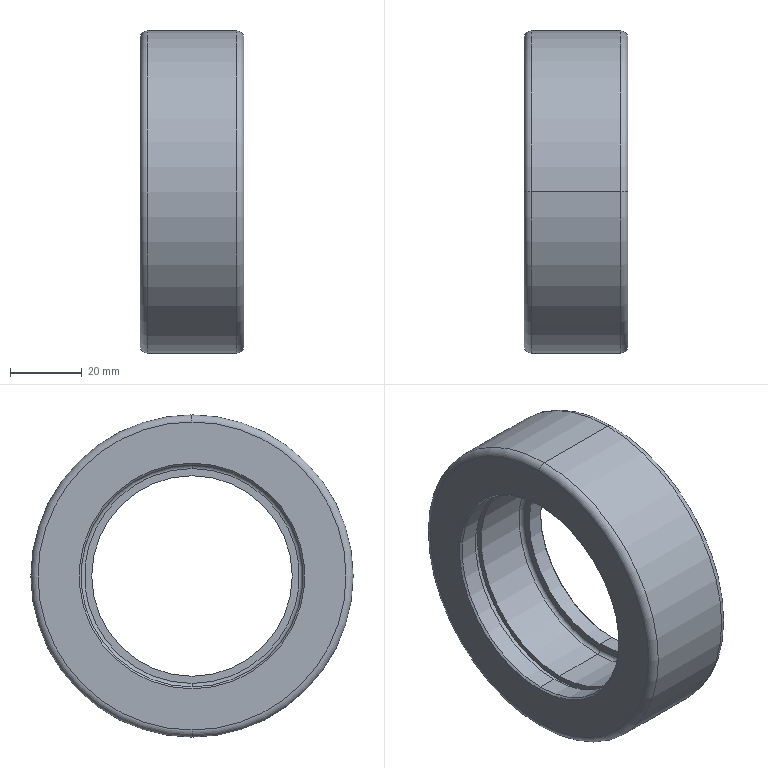Part | STEP file | PN_0001-01-11 Guide wheel B | 1 solid | 25 faces | box 29 x 90 x 90 mm | volume 98573 mm3 | cylinder 10 | torus 6 | plane 5 | cone 4 | commonest cylinder face diameters 62 x4 56 x2 65 x2 90 x2
STEP:
#1=CARTESIAN_POINT('',(0.5,0.,-31.));
#2=VERTEX_POINT('',#1);
#3=CARTESIAN_POINT('',(0.5,0.,31.));
#4=VERTEX_POINT('',#3);
#5=CARTESIAN_POINT('',(0.5,0.,0.));
#6=DIRECTION('',(-1.,0.,0.));
#7=DIRECTION('',(0.,0.,-1.));
#8=AXIS2_PLACEMENT_3D('',#5,#6,#7);
#9=CIRCLE('',#8,31.);
#10=EDGE_CURVE('',#2,#4,#9,.T.);
#11=ORIENTED_EDGE('',*,*,#10,.F.);
#12=CARTESIAN_POINT('',(0.,0.,-31.5));
#13=VERTEX_POINT('',#12);
#14=CARTESIAN_POINT('',(0.5,0.,-31.));
#15=DIRECTION('',(-0.7071,0.,-0.7071));
#16=VECTOR('',#15,1000.);
#17=LINE('',#14,#16);
#18=EDGE_CURVE('',#2,#13,#17,.T.);
#19=ORIENTED_EDGE('',*,*,#18,.T.);
#20=CARTESIAN_POINT('',(0.,0.,31.5));
#21=VERTEX_POINT('',#20);
#22=CARTESIAN_POINT('',(0.,0.,0.));
#23=DIRECTION('',(1.,0.,0.));
#24=DIRECTION('',(0.,0.,-1.));
#25=AXIS2_PLACEMENT_3D('',#22,#23,#24);
#26=CIRCLE('',#25,31.5);
#27=EDGE_CURVE('',#21,#13,#26,.T.);
#28=ORIENTED_EDGE('',*,*,#27,.F.);
#29=CARTESIAN_POINT('',(0.5,0.,31.));
#30=DIRECTION('',(-0.7071,0.,0.7071));
#31=VECTOR('',#30,1000.);
#32=LINE('',#29,#31);
#33=EDGE_CURVE('',#4,#21,#32,.T.);
#34=ORIENTED_EDGE('',*,*,#33,.F.);
#35=EDGE_LOOP('',(#11,#19,#28,#34));
#36=FACE_OUTER_BOUND('',#35,.T.);
#37=CARTESIAN_POINT('',(0.5,0.,0.));
#38=DIRECTION('',(-1.,0.,0.));
#39=DIRECTION('',(0.,0.,1.));
#40=AXIS2_PLACEMENT_3D('',#37,#38,#39);
#41=CONICAL_SURFACE('',#40,31.,0.7854);
#42=ADVANCED_FACE('',(#36),#41,.F.);
#43=CARTESIAN_POINT('',(28.5,0.,28.));
#44=VERTEX_POINT('',#43);
#45=CARTESIAN_POINT('',(28.5,0.,-28.));
#46=VERTEX_POINT('',#45);
#47=CARTESIAN_POINT('',(28.5,0.,0.));
#48=DIRECTION('',(1.,0.,0.));
#49=DIRECTION('',(0.,0.,1.));
#50=AXIS2_PLACEMENT_3D('',#47,#48,#49);
#51=CIRCLE('',#50,28.);
#52=EDGE_CURVE('',#44,#46,#51,.T.);
#53=ORIENTED_EDGE('',*,*,#52,.F.);
#54=CARTESIAN_POINT('',(29.,0.,28.5));
#55=VERTEX_POINT('',#54);
#56=CARTESIAN_POINT('',(29.,0.,28.5));
#57=DIRECTION('',(0.7071,0.,0.7071));
#58=VECTOR('',#57,1000.);
#59=LINE('',#56,#58);
#60=EDGE_CURVE('',#44,#55,#59,.T.);
#61=ORIENTED_EDGE('',*,*,#60,.T.);
#62=CARTESIAN_POINT('',(29.,0.,-28.5));
#63=VERTEX_POINT('',#62);
#64=CARTESIAN_POINT('',(29.,0.,0.));
#65=DIRECTION('',(-1.,0.,0.));
#66=DIRECTION('',(0.,0.,1.));
#67=AXIS2_PLACEMENT_3D('',#64,#65,#66);
#68=CIRCLE('',#67,28.5);
#69=EDGE_CURVE('',#63,#55,#68,.T.);
#70=ORIENTED_EDGE('',*,*,#69,.F.);
#71=CARTESIAN_POINT('',(29.,0.,-28.5));
#72=DIRECTION('',(0.7071,0.,-0.7071));
#73=VECTOR('',#72,1000.);
#74=LINE('',#71,#73);
#75=EDGE_CURVE('',#46,#63,#74,.T.);
#76=ORIENTED_EDGE('',*,*,#75,.F.);
#77=EDGE_LOOP('',(#53,#61,#70,#76));
#78=FACE_OUTER_BOUND('',#77,.T.);
#79=CARTESIAN_POINT('',(29.,0.,0.));
#80=DIRECTION('',(1.,0.,0.));
#81=DIRECTION('',(0.,0.,-1.));
#82=AXIS2_PLACEMENT_3D('',#79,#80,#81);
#83=CONICAL_SURFACE('',#82,28.5,0.7854);
#84=ADVANCED_FACE('',(#78),#83,.F.);
#85=CARTESIAN_POINT('',(29.,0.,-43.));
#86=VERTEX_POINT('',#85);
#87=CARTESIAN_POINT('',(29.,0.,43.));
#88=VERTEX_POINT('',#87);
#89=CARTESIAN_POINT('',(29.,0.,0.));
#90=DIRECTION('',(1.,0.,0.));
#91=DIRECTION('',(0.,0.,1.));
#92=AXIS2_PLACEMENT_3D('',#89,#90,#91);
#93=CIRCLE('',#92,43.);
#94=EDGE_CURVE('',#86,#88,#93,.T.);
#95=ORIENTED_EDGE('',*,*,#94,.F.);
#96=CARTESIAN_POINT('',(27.,0.,-45.));
#97=VERTEX_POINT('',#96);
#98=CARTESIAN_POINT('',(27.,0.,-43.));
#99=DIRECTION('',(0.,1.,0.));
#100=DIRECTION('',(0.,0.,1.));
#101=AXIS2_PLACEMENT_3D('',#98,#99,#100);
#102=CIRCLE('',#101,2.);
#103=EDGE_CURVE('',#86,#97,#102,.T.);
#104=ORIENTED_EDGE('',*,*,#103,.T.);
#105=CARTESIAN_POINT('',(27.,0.,45.));
#106=VERTEX_POINT('',#105);
#107=CARTESIAN_POINT('',(27.,0.,0.));
#108=DIRECTION('',(-1.,0.,0.));
#109=DIRECTION('',(0.,0.,1.));
#110=AXIS2_PLACEMENT_3D('',#107,#108,#109);
#111=CIRCLE('',#110,45.);
#112=EDGE_CURVE('',#106,#97,#111,.T.);
#113=ORIENTED_EDGE('',*,*,#112,.F.);
#114=CARTESIAN_POINT('',(27.,0.,43.));
#115=DIRECTION('',(0.,-1.,0.));
#116=DIRECTION('',(0.,0.,-1.));
#117=AXIS2_PLACEMENT_3D('',#114,#115,#116);
#118=CIRCLE('',#117,2.);
#119=EDGE_CURVE('',#88,#106,#118,.T.);
#120=ORIENTED_EDGE('',*,*,#119,.F.);
#121=EDGE_LOOP('',(#95,#104,#113,#120));
#122=FACE_OUTER_BOUND('',#121,.T.);
#123=CARTESIAN_POINT('',(27.,0.,0.));
#124=DIRECTION('',(-1.,0.,0.));
#125=DIRECTION('',(0.,0.,1.));
#126=AXIS2_PLACEMENT_3D('',#123,#124,#125);
#127=TOROIDAL_SURFACE('',#126,43.,2.);
#128=ADVANCED_FACE('',(#122),#127,.T.);
#129=CARTESIAN_POINT('',(0.,0.,43.));
#130=VERTEX_POINT('',#129);
#131=CARTESIAN_POINT('',(0.,0.,-43.));
#132=VERTEX_POINT('',#131);
#133=CARTESIAN_POINT('',(0.,0.,0.));
#134=DIRECTION('',(-1.,0.,0.));
#135=DIRECTION('',(0.,0.,-1.));
#136=AXIS2_PLACEMENT_3D('',#133,#134,#135);
#137=CIRCLE('',#136,43.);
#138=EDGE_CURVE('',#130,#132,#137,.T.);
#139=ORIENTED_EDGE('',*,*,#138,.F.);
#140=CARTESIAN_POINT('',(2.,0.,45.));
#141=VERTEX_POINT('',#140);
#142=CARTESIAN_POINT('',(2.,0.,43.));
#143=DIRECTION('',(0.,1.,0.));
#144=DIRECTION('',(0.,0.,1.));
#145=AXIS2_PLACEMENT_3D('',#142,#143,#144);
#146=CIRCLE('',#145,2.);
#147=EDGE_CURVE('',#130,#141,#146,.T.);
#148=ORIENTED_EDGE('',*,*,#147,.T.);
#149=CARTESIAN_POINT('',(2.,0.,-45.));
#150=VERTEX_POINT('',#149);
#151=CARTESIAN_POINT('',(2.,0.,0.));
#152=DIRECTION('',(1.,0.,0.));
#153=DIRECTION('',(0.,0.,-1.));
#154=AXIS2_PLACEMENT_3D('',#151,#152,#153);
#155=CIRCLE('',#154,45.);
#156=EDGE_CURVE('',#150,#141,#155,.T.);
#157=ORIENTED_EDGE('',*,*,#156,.F.);
#158=CARTESIAN_POINT('',(2.,0.,-43.));
#159=DIRECTION('',(0.,-1.,0.));
#160=DIRECTION('',(0.,0.,-1.));
#161=AXIS2_PLACEMENT_3D('',#158,#159,#160);
#162=CIRCLE('',#161,2.);
#163=EDGE_CURVE('',#132,#150,#162,.T.);
#164=ORIENTED_EDGE('',*,*,#163,.F.);
#165=EDGE_LOOP('',(#139,#148,#157,#164));
#166=FACE_OUTER_BOUND('',#165,.T.);
#167=CARTESIAN_POINT('',(2.,0.,0.));
#168=DIRECTION('',(1.,0.,0.));
#169=DIRECTION('',(0.,0.,-1.));
#170=AXIS2_PLACEMENT_3D('',#167,#168,#169);
#171=TOROIDAL_SURFACE('',#170,43.,2.);
#172=ADVANCED_FACE('',(#166),#171,.T.);
#173=ORIENTED_EDGE('',*,*,#52,.T.);
#174=CARTESIAN_POINT('',(24.,0.,-28.));
#175=VERTEX_POINT('',#174);
#176=CARTESIAN_POINT('',(0.,0.,-28.));
#177=DIRECTION('',(-1.,0.,0.));
#178=VECTOR('',#177,1000.);
#179=LINE('',#176,#178);
#180=EDGE_CURVE('',#46,#175,#179,.T.);
#181=ORIENTED_EDGE('',*,*,#180,.T.);
#182=CARTESIAN_POINT('',(24.,0.,28.));
#183=VERTEX_POINT('',#182);
#184=CARTESIAN_POINT('',(24.,0.,0.));
#185=DIRECTION('',(-1.,0.,0.));
#186=DIRECTION('',(0.,0.,1.));
#187=AXIS2_PLACEMENT_3D('',#184,#185,#186);
#188=CIRCLE('',#187,28.);
#189=EDGE_CURVE('',#175,#183,#188,.T.);
#190=ORIENTED_EDGE('',*,*,#189,.T.);
#191=CARTESIAN_POINT('',(0.,0.,28.));
#192=DIRECTION('',(-1.,0.,0.));
#193=VECTOR('',#192,1000.);
#194=LINE('',#191,#193);
#195=EDGE_CURVE('',#44,#183,#194,.T.);
#196=ORIENTED_EDGE('',*,*,#195,.F.);
#197=EDGE_LOOP('',(#173,#181,#190,#196));
#198=FACE_OUTER_BOUND('',#197,.T.);
#199=CARTESIAN_POINT('',(0.,0.,0.));
#200=DIRECTION('',(-1.,0.,0.));
#201=DIRECTION('',(0.,0.,1.));
#202=AXIS2_PLACEMENT_3D('',#199,#200,#201);
#203=CYLINDRICAL_SURFACE('',#202,28.);
#204=ADVANCED_FACE('',(#198),#203,.F.);
#205=ORIENTED_EDGE('',*,*,#112,.T.);
#206=CARTESIAN_POINT('',(0.,0.,-45.));
#207=DIRECTION('',(-1.,0.,0.));
#208=VECTOR('',#207,1000.);
#209=LINE('',#206,#208);
#210=EDGE_CURVE('',#97,#150,#209,.T.);
#211=ORIENTED_EDGE('',*,*,#210,.T.);
#212=ORIENTED_EDGE('',*,*,#156,.T.);
#213=CARTESIAN_POINT('',(0.,0.,45.));
#214=DIRECTION('',(-1.,0.,0.));
#215=VECTOR('',#214,1000.);
#216=LINE('',#213,#215);
#217=EDGE_CURVE('',#106,#141,#216,.T.);
#218=ORIENTED_EDGE('',*,*,#217,.F.);
#219=EDGE_LOOP('',(#205,#211,#212,#218));
#220=FACE_OUTER_BOUND('',#219,.T.);
#221=CARTESIAN_POINT('',(0.,0.,0.));
#222=DIRECTION('',(-1.,0.,0.));
#223=DIRECTION('',(0.,0.,1.));
#224=AXIS2_PLACEMENT_3D('',#221,#222,#223);
#225=CYLINDRICAL_SURFACE('',#224,45.);
#226=ADVANCED_FACE('',(#220),#225,.T.);
#227=CARTESIAN_POINT('',(5.8,0.,-31.));
#228=VERTEX_POINT('',#227);
#229=CARTESIAN_POINT('',(5.8,0.,31.));
#230=VERTEX_POINT('',#229);
#231=CARTESIAN_POINT('',(5.8,0.,0.));
#232=DIRECTION('',(-1.,0.,0.));
#233=DIRECTION('',(0.,0.,1.));
#234=AXIS2_PLACEMENT_3D('',#231,#232,#233);
#235=CIRCLE('',#234,31.);
#236=EDGE_CURVE('',#228,#230,#235,.T.);
#237=ORIENTED_EDGE('',*,*,#236,.F.);
#238=CARTESIAN_POINT('',(0.,0.,-31.));
#239=DIRECTION('',(-1.,0.,0.));
#240=VECTOR('',#239,1000.);
#241=LINE('',#238,#240);
#242=EDGE_CURVE('',#228,#2,#241,.T.);
#243=ORIENTED_EDGE('',*,*,#242,.T.);
#244=ORIENTED_EDGE('',*,*,#10,.T.);
#245=CARTESIAN_POINT('',(0.,0.,31.));
#246=DIRECTION('',(-1.,0.,0.));
#247=VECTOR('',#246,1000.);
#248=LINE('',#245,#247);
#249=EDGE_CURVE('',#230,#4,#248,.T.);
#250=ORIENTED_EDGE('',*,*,#249,.F.);
#251=EDGE_LOOP('',(#237,#243,#244,#250));
#252=FACE_OUTER_BOUND('',#251,.T.);
#253=CARTESIAN_POINT('',(0.,0.,0.));
#254=DIRECTION('',(-1.,0.,0.));
#255=DIRECTION('',(0.,0.,1.));
#256=AXIS2_PLACEMENT_3D('',#253,#254,#255);
#257=CYLINDRICAL_SURFACE('',#256,31.);
#258=ADVANCED_FACE('',(#252),#257,.F.);
#259=CARTESIAN_POINT('',(8.,0.,-32.5));
#260=VERTEX_POINT('',#259);
#261=CARTESIAN_POINT('',(8.,0.,32.5));
#262=VERTEX_POINT('',#261);
#263=CARTESIAN_POINT('',(8.,0.,0.));
#264=DIRECTION('',(-1.,0.,0.));
#265=DIRECTION('',(0.,0.,1.));
#266=AXIS2_PLACEMENT_3D('',#263,#264,#265);
#267=CIRCLE('',#266,32.5);
#268=EDGE_CURVE('',#260,#262,#267,.T.);
#269=ORIENTED_EDGE('',*,*,#268,.F.);
#270=CARTESIAN_POINT('',(5.8,0.,-32.5));
#271=VERTEX_POINT('',#270);
#272=CARTESIAN_POINT('',(0.,0.,-32.5));
#273=DIRECTION('',(-1.,0.,0.));
#274=VECTOR('',#273,1000.);
#275=LINE('',#272,#274);
#276=EDGE_CURVE('',#260,#271,#275,.T.);
#277=ORIENTED_EDGE('',*,*,#276,.T.);
#278=CARTESIAN_POINT('',(5.8,0.,32.5));
#279=VERTEX_POINT('',#278);
#280=CARTESIAN_POINT('',(5.8,0.,0.));
#281=DIRECTION('',(-1.,0.,0.));
#282=DIRECTION('',(0.,0.,1.));
#283=AXIS2_PLACEMENT_3D('',#280,#281,#282);
#284=CIRCLE('',#283,32.5);
#285=EDGE_CURVE('',#271,#279,#284,.T.);
#286=ORIENTED_EDGE('',*,*,#285,.T.);
#287=CARTESIAN_POINT('',(0.,0.,32.5));
#288=DIRECTION('',(-1.,0.,0.));
#289=VECTOR('',#288,1000.);
#290=LINE('',#287,#289);
#291=EDGE_CURVE('',#262,#279,#290,.T.);
#292=ORIENTED_EDGE('',*,*,#291,.F.);
#293=EDGE_LOOP('',(#269,#277,#286,#292));
#294=FACE_OUTER_BOUND('',#293,.T.);
#295=CARTESIAN_POINT('',(0.,0.,0.));
#296=DIRECTION('',(-1.,0.,0.));
#297=DIRECTION('',(0.,0.,1.));
#298=AXIS2_PLACEMENT_3D('',#295,#296,#297);
#299=CYLINDRICAL_SURFACE('',#298,32.5);
#300=ADVANCED_FACE('',(#294),#299,.F.);
#301=CARTESIAN_POINT('',(23.,0.,-31.));
#302=VERTEX_POINT('',#301);
#303=CARTESIAN_POINT('',(23.,0.,31.));
#304=VERTEX_POINT('',#303);
#305=CARTESIAN_POINT('',(23.,0.,0.));
#306=DIRECTION('',(-1.,0.,0.));
#307=DIRECTION('',(0.,0.,1.));
#308=AXIS2_PLACEMENT_3D('',#305,#306,#307);
#309=CIRCLE('',#308,31.);
#310=EDGE_CURVE('',#302,#304,#309,.T.);
#311=ORIENTED_EDGE('',*,*,#310,.F.);
#312=CARTESIAN_POINT('',(8.,0.,-31.));
#313=VERTEX_POINT('',#312);
#314=CARTESIAN_POINT('',(0.,0.,-31.));
#315=DIRECTION('',(-1.,0.,0.));
#316=VECTOR('',#315,1000.);
#317=LINE('',#314,#316);
#318=EDGE_CURVE('',#302,#313,#317,.T.);
#319=ORIENTED_EDGE('',*,*,#318,.T.);
#320=CARTESIAN_POINT('',(8.,0.,31.));
#321=VERTEX_POINT('',#320);
#322=CARTESIAN_POINT('',(8.,0.,0.));
#323=DIRECTION('',(-1.,0.,0.));
#324=DIRECTION('',(0.,0.,1.));
#325=AXIS2_PLACEMENT_3D('',#322,#323,#324);
#326=CIRCLE('',#325,31.);
#327=EDGE_CURVE('',#313,#321,#326,.T.);
#328=ORIENTED_EDGE('',*,*,#327,.T.);
#329=CARTESIAN_POINT('',(0.,0.,31.));
#330=DIRECTION('',(-1.,0.,0.));
#331=VECTOR('',#330,1000.);
#332=LINE('',#329,#331);
#333=EDGE_CURVE('',#304,#321,#332,.T.);
#334=ORIENTED_EDGE('',*,*,#333,.F.);
#335=EDGE_LOOP('',(#311,#319,#328,#334));
#336=FACE_OUTER_BOUND('',#335,.T.);
#337=CARTESIAN_POINT('',(0.,0.,0.));
#338=DIRECTION('',(-1.,0.,0.));
#339=DIRECTION('',(0.,0.,1.));
#340=AXIS2_PLACEMENT_3D('',#337,#338,#339);
#341=CYLINDRICAL_SURFACE('',#340,31.);
#342=ADVANCED_FACE('',(#336),#341,.F.);
#343=CARTESIAN_POINT('',(24.,0.,-30.));
#344=VERTEX_POINT('',#343);
#345=CARTESIAN_POINT('',(24.,0.,30.));
#346=VERTEX_POINT('',#345);
#347=CARTESIAN_POINT('',(24.,0.,0.));
#348=DIRECTION('',(-1.,0.,0.));
#349=DIRECTION('',(0.,0.,1.));
#350=AXIS2_PLACEMENT_3D('',#347,#348,#349);
#351=CIRCLE('',#350,30.);
#352=EDGE_CURVE('',#344,#346,#351,.T.);
#353=ORIENTED_EDGE('',*,*,#352,.F.);
#354=CARTESIAN_POINT('',(23.,0.,-30.));
#355=DIRECTION('',(0.,1.,0.));
#356=DIRECTION('',(0.,0.,1.));
#357=AXIS2_PLACEMENT_3D('',#354,#355,#356);
#358=CIRCLE('',#357,1.);
#359=EDGE_CURVE('',#344,#302,#358,.T.);
#360=ORIENTED_EDGE('',*,*,#359,.T.);
#361=ORIENTED_EDGE('',*,*,#310,.T.);
#362=CARTESIAN_POINT('',(23.,0.,30.));
#363=DIRECTION('',(0.,-1.,0.));
#364=DIRECTION('',(0.,0.,-1.));
#365=AXIS2_PLACEMENT_3D('',#362,#363,#364);
#366=CIRCLE('',#365,1.);
#367=EDGE_CURVE('',#346,#304,#366,.T.);
#368=ORIENTED_EDGE('',*,*,#367,.F.);
#369=EDGE_LOOP('',(#353,#360,#361,#368));
#370=FACE_OUTER_BOUND('',#369,.T.);
#371=CARTESIAN_POINT('',(23.,0.,0.));
#372=DIRECTION('',(-1.,0.,0.));
#373=DIRECTION('',(0.,0.,1.));
#374=AXIS2_PLACEMENT_3D('',#371,#372,#373);
#375=TOROIDAL_SURFACE('',#374,30.,1.);
#376=ADVANCED_FACE('',(#370),#375,.F.);
#377=ORIENTED_EDGE('',*,*,#359,.F.);
#378=CARTESIAN_POINT('',(24.,0.,0.));
#379=DIRECTION('',(-1.,0.,0.));
#380=DIRECTION('',(0.,0.,1.));
#381=AXIS2_PLACEMENT_3D('',#378,#379,#380);
#382=CIRCLE('',#381,30.);
#383=EDGE_CURVE('',#346,#344,#382,.T.);
#384=ORIENTED_EDGE('',*,*,#383,.F.);
#385=ORIENTED_EDGE('',*,*,#367,.T.);
#386=CARTESIAN_POINT('',(23.,0.,0.));
#387=DIRECTION('',(-1.,0.,0.));
#388=DIRECTION('',(0.,0.,1.));
#389=AXIS2_PLACEMENT_3D('',#386,#387,#388);
#390=CIRCLE('',#389,31.);
#391=EDGE_CURVE('',#304,#302,#390,.T.);
#392=ORIENTED_EDGE('',*,*,#391,.T.);
#393=EDGE_LOOP('',(#377,#384,#385,#392));
#394=FACE_OUTER_BOUND('',#393,.T.);
#395=CARTESIAN_POINT('',(23.,0.,0.));
#396=DIRECTION('',(-1.,0.,0.));
#397=DIRECTION('',(0.,0.,1.));
#398=AXIS2_PLACEMENT_3D('',#395,#396,#397);
#399=TOROIDAL_SURFACE('',#398,30.,1.);
#400=ADVANCED_FACE('',(#394),#399,.F.);
#401=ORIENTED_EDGE('',*,*,#318,.F.);
#402=ORIENTED_EDGE('',*,*,#391,.F.);
#403=ORIENTED_EDGE('',*,*,#333,.T.);
#404=CARTESIAN_POINT('',(8.,0.,0.));
#405=DIRECTION('',(-1.,0.,0.));
#406=DIRECTION('',(0.,0.,1.));
#407=AXIS2_PLACEMENT_3D('',#404,#405,#406);
#408=CIRCLE('',#407,31.);
#409=EDGE_CURVE('',#321,#313,#408,.T.);
#410=ORIENTED_EDGE('',*,*,#409,.T.);
#411=EDGE_LOOP('',(#401,#402,#403,#410));
#412=FACE_OUTER_BOUND('',#411,.T.);
#413=CARTESIAN_POINT('',(0.,0.,0.));
#414=DIRECTION('',(-1.,0.,0.));
#415=DIRECTION('',(0.,0.,1.));
#416=AXIS2_PLACEMENT_3D('',#413,#414,#415);
#417=CYLINDRICAL_SURFACE('',#416,31.);
#418=ADVANCED_FACE('',(#412),#417,.F.);
#419=ORIENTED_EDGE('',*,*,#409,.F.);
#420=ORIENTED_EDGE('',*,*,#327,.F.);
#421=EDGE_LOOP('',(#419,#420));
#422=FACE_BOUND('',#421,.T.);
#423=CARTESIAN_POINT('',(8.,0.,0.));
#424=DIRECTION('',(-1.,0.,0.));
#425=DIRECTION('',(0.,0.,1.));
#426=AXIS2_PLACEMENT_3D('',#423,#424,#425);
#427=CIRCLE('',#426,32.5);
#428=EDGE_CURVE('',#262,#260,#427,.T.);
#429=ORIENTED_EDGE('',*,*,#428,.T.);
#430=ORIENTED_EDGE('',*,*,#268,.T.);
#431=EDGE_LOOP('',(#429,#430));
#432=FACE_OUTER_BOUND('',#431,.T.);
#433=CARTESIAN_POINT('',(8.,32.5,0.));
#434=DIRECTION('',(1.,0.,0.));
#435=DIRECTION('',(0.,0.,-1.));
#436=AXIS2_PLACEMENT_3D('',#433,#434,#435);
#437=PLANE('',#436);
#438=ADVANCED_FACE('',(#422,#432),#437,.F.);
#439=ORIENTED_EDGE('',*,*,#276,.F.);
#440=ORIENTED_EDGE('',*,*,#428,.F.);
#441=ORIENTED_EDGE('',*,*,#291,.T.);
#442=CARTESIAN_POINT('',(5.8,0.,0.));
#443=DIRECTION('',(-1.,0.,0.));
#444=DIRECTION('',(0.,0.,1.));
#445=AXIS2_PLACEMENT_3D('',#442,#443,#444);
#446=CIRCLE('',#445,32.5);
#447=EDGE_CURVE('',#279,#271,#446,.T.);
#448=ORIENTED_EDGE('',*,*,#447,.T.);
#449=EDGE_LOOP('',(#439,#440,#441,#448));
#450=FACE_OUTER_BOUND('',#449,.T.);
#451=CARTESIAN_POINT('',(0.,0.,0.));
#452=DIRECTION('',(-1.,0.,0.));
#453=DIRECTION('',(0.,0.,1.));
#454=AXIS2_PLACEMENT_3D('',#451,#452,#453);
#455=CYLINDRICAL_SURFACE('',#454,32.5);
#456=ADVANCED_FACE('',(#450),#455,.F.);
#457=ORIENTED_EDGE('',*,*,#447,.F.);
#458=ORIENTED_EDGE('',*,*,#285,.F.);
#459=EDGE_LOOP('',(#457,#458));
#460=FACE_OUTER_BOUND('',#459,.T.);
#461=CARTESIAN_POINT('',(5.8,0.,0.));
#462=DIRECTION('',(-1.,0.,0.));
#463=DIRECTION('',(0.,0.,1.));
#464=AXIS2_PLACEMENT_3D('',#461,#462,#463);
#465=CIRCLE('',#464,31.);
#466=EDGE_CURVE('',#230,#228,#465,.T.);
#467=ORIENTED_EDGE('',*,*,#466,.T.);
#468=ORIENTED_EDGE('',*,*,#236,.T.);
#469=EDGE_LOOP('',(#467,#468));
#470=FACE_BOUND('',#469,.T.);
#471=CARTESIAN_POINT('',(5.8,31.,0.));
#472=DIRECTION('',(-1.,0.,0.));
#473=DIRECTION('',(0.,0.,1.));
#474=AXIS2_PLACEMENT_3D('',#471,#472,#473);
#475=PLANE('',#474);
#476=ADVANCED_FACE('',(#460,#470),#475,.F.);
#477=ORIENTED_EDGE('',*,*,#242,.F.);
#478=ORIENTED_EDGE('',*,*,#466,.F.);
#479=ORIENTED_EDGE('',*,*,#249,.T.);
#480=CARTESIAN_POINT('',(0.5,0.,0.));
#481=DIRECTION('',(-1.,0.,0.));
#482=DIRECTION('',(0.,0.,-1.));
#483=AXIS2_PLACEMENT_3D('',#480,#481,#482);
#484=CIRCLE('',#483,31.);
#485=EDGE_CURVE('',#4,#2,#484,.T.);
#486=ORIENTED_EDGE('',*,*,#485,.T.);
#487=EDGE_LOOP('',(#477,#478,#479,#486));
#488=FACE_OUTER_BOUND('',#487,.T.);
#489=CARTESIAN_POINT('',(0.,0.,0.));
#490=DIRECTION('',(-1.,0.,0.));
#491=DIRECTION('',(0.,0.,1.));
#492=AXIS2_PLACEMENT_3D('',#489,#490,#491);
#493=CYLINDRICAL_SURFACE('',#492,31.);
#494=ADVANCED_FACE('',(#488),#493,.F.);
#495=ORIENTED_EDGE('',*,*,#27,.T.);
#496=CARTESIAN_POINT('',(0.,0.,0.));
#497=DIRECTION('',(1.,0.,0.));
#498=DIRECTION('',(0.,0.,-1.));
#499=AXIS2_PLACEMENT_3D('',#496,#497,#498);
#500=CIRCLE('',#499,31.5);
#501=EDGE_CURVE('',#13,#21,#500,.T.);
#502=ORIENTED_EDGE('',*,*,#501,.T.);
#503=EDGE_LOOP('',(#495,#502));
#504=FACE_BOUND('',#503,.T.);
#505=CARTESIAN_POINT('',(0.,0.,0.));
#506=DIRECTION('',(-1.,0.,0.));
#507=DIRECTION('',(0.,0.,-1.));
#508=AXIS2_PLACEMENT_3D('',#505,#506,#507);
#509=CIRCLE('',#508,43.);
#510=EDGE_CURVE('',#132,#130,#509,.T.);
#511=ORIENTED_EDGE('',*,*,#510,.T.);
#512=ORIENTED_EDGE('',*,*,#138,.T.);
#513=EDGE_LOOP('',(#511,#512));
#514=FACE_OUTER_BOUND('',#513,.T.);
#515=CARTESIAN_POINT('',(0.,45.,0.));
#516=DIRECTION('',(1.,0.,0.));
#517=DIRECTION('',(0.,0.,-1.));
#518=AXIS2_PLACEMENT_3D('',#515,#516,#517);
#519=PLANE('',#518);
#520=ADVANCED_FACE('',(#504,#514),#519,.F.);
#521=ORIENTED_EDGE('',*,*,#210,.F.);
#522=CARTESIAN_POINT('',(27.,0.,0.));
#523=DIRECTION('',(-1.,0.,0.));
#524=DIRECTION('',(0.,0.,1.));
#525=AXIS2_PLACEMENT_3D('',#522,#523,#524);
#526=CIRCLE('',#525,45.);
#527=EDGE_CURVE('',#97,#106,#526,.T.);
#528=ORIENTED_EDGE('',*,*,#527,.T.);
#529=ORIENTED_EDGE('',*,*,#217,.T.);
#530=CARTESIAN_POINT('',(2.,0.,0.));
#531=DIRECTION('',(1.,0.,0.));
#532=DIRECTION('',(0.,0.,-1.));
#533=AXIS2_PLACEMENT_3D('',#530,#531,#532);
#534=CIRCLE('',#533,45.);
#535=EDGE_CURVE('',#141,#150,#534,.T.);
#536=ORIENTED_EDGE('',*,*,#535,.T.);
#537=EDGE_LOOP('',(#521,#528,#529,#536));
#538=FACE_OUTER_BOUND('',#537,.T.);
#539=CARTESIAN_POINT('',(0.,0.,0.));
#540=DIRECTION('',(-1.,0.,0.));
#541=DIRECTION('',(0.,0.,1.));
#542=AXIS2_PLACEMENT_3D('',#539,#540,#541);
#543=CYLINDRICAL_SURFACE('',#542,45.);
#544=ADVANCED_FACE('',(#538),#543,.T.);
#545=ORIENTED_EDGE('',*,*,#69,.T.);
#546=CARTESIAN_POINT('',(29.,0.,0.));
#547=DIRECTION('',(-1.,0.,0.));
#548=DIRECTION('',(0.,0.,1.));
#549=AXIS2_PLACEMENT_3D('',#546,#547,#548);
#550=CIRCLE('',#549,28.5);
#551=EDGE_CURVE('',#55,#63,#550,.T.);
#552=ORIENTED_EDGE('',*,*,#551,.T.);
#553=EDGE_LOOP('',(#545,#552));
#554=FACE_BOUND('',#553,.T.);
#555=CARTESIAN_POINT('',(29.,0.,0.));
#556=DIRECTION('',(1.,0.,0.));
#557=DIRECTION('',(0.,0.,1.));
#558=AXIS2_PLACEMENT_3D('',#555,#556,#557);
#559=CIRCLE('',#558,43.);
#560=EDGE_CURVE('',#88,#86,#559,.T.);
#561=ORIENTED_EDGE('',*,*,#560,.T.);
#562=ORIENTED_EDGE('',*,*,#94,.T.);
#563=EDGE_LOOP('',(#561,#562));
#564=FACE_OUTER_BOUND('',#563,.T.);
#565=CARTESIAN_POINT('',(29.,28.,0.));
#566=DIRECTION('',(-1.,0.,0.));
#567=DIRECTION('',(0.,0.,1.));
#568=AXIS2_PLACEMENT_3D('',#565,#566,#567);
#569=PLANE('',#568);
#570=ADVANCED_FACE('',(#554,#564),#569,.F.);
#571=ORIENTED_EDGE('',*,*,#180,.F.);
#572=CARTESIAN_POINT('',(28.5,0.,0.));
#573=DIRECTION('',(1.,0.,0.));
#574=DIRECTION('',(0.,0.,1.));
#575=AXIS2_PLACEMENT_3D('',#572,#573,#574);
#576=CIRCLE('',#575,28.);
#577=EDGE_CURVE('',#46,#44,#576,.T.);
#578=ORIENTED_EDGE('',*,*,#577,.T.);
#579=ORIENTED_EDGE('',*,*,#195,.T.);
#580=CARTESIAN_POINT('',(24.,0.,0.));
#581=DIRECTION('',(-1.,0.,0.));
#582=DIRECTION('',(0.,0.,1.));
#583=AXIS2_PLACEMENT_3D('',#580,#581,#582);
#584=CIRCLE('',#583,28.);
#585=EDGE_CURVE('',#183,#175,#584,.T.);
#586=ORIENTED_EDGE('',*,*,#585,.T.);
#587=EDGE_LOOP('',(#571,#578,#579,#586));
#588=FACE_OUTER_BOUND('',#587,.T.);
#589=CARTESIAN_POINT('',(0.,0.,0.));
#590=DIRECTION('',(-1.,0.,0.));
#591=DIRECTION('',(0.,0.,1.));
#592=AXIS2_PLACEMENT_3D('',#589,#590,#591);
#593=CYLINDRICAL_SURFACE('',#592,28.);
#594=ADVANCED_FACE('',(#588),#593,.F.);
#595=ORIENTED_EDGE('',*,*,#585,.F.);
#596=ORIENTED_EDGE('',*,*,#189,.F.);
#597=EDGE_LOOP('',(#595,#596));
#598=FACE_BOUND('',#597,.T.);
#599=ORIENTED_EDGE('',*,*,#383,.T.);
#600=ORIENTED_EDGE('',*,*,#352,.T.);
#601=EDGE_LOOP('',(#599,#600));
#602=FACE_OUTER_BOUND('',#601,.T.);
#603=CARTESIAN_POINT('',(24.,30.,0.));
#604=DIRECTION('',(1.,0.,0.));
#605=DIRECTION('',(0.,0.,-1.));
#606=AXIS2_PLACEMENT_3D('',#603,#604,#605);
#607=PLANE('',#606);
#608=ADVANCED_FACE('',(#598,#602),#607,.F.);
#609=ORIENTED_EDGE('',*,*,#147,.F.);
#610=ORIENTED_EDGE('',*,*,#510,.F.);
#611=ORIENTED_EDGE('',*,*,#163,.T.);
#612=ORIENTED_EDGE('',*,*,#535,.F.);
#613=EDGE_LOOP('',(#609,#610,#611,#612));
#614=FACE_OUTER_BOUND('',#613,.T.);
#615=CARTESIAN_POINT('',(2.,0.,0.));
#616=DIRECTION('',(1.,0.,0.));
#617=DIRECTION('',(0.,0.,-1.));
#618=AXIS2_PLACEMENT_3D('',#615,#616,#617);
#619=TOROIDAL_SURFACE('',#618,43.,2.);
#620=ADVANCED_FACE('',(#614),#619,.T.);
#621=ORIENTED_EDGE('',*,*,#103,.F.);
#622=ORIENTED_EDGE('',*,*,#560,.F.);
#623=ORIENTED_EDGE('',*,*,#119,.T.);
#624=ORIENTED_EDGE('',*,*,#527,.F.);
#625=EDGE_LOOP('',(#621,#622,#623,#624));
#626=FACE_OUTER_BOUND('',#625,.T.);
#627=CARTESIAN_POINT('',(27.,0.,0.));
#628=DIRECTION('',(-1.,0.,0.));
#629=DIRECTION('',(0.,0.,1.));
#630=AXIS2_PLACEMENT_3D('',#627,#628,#629);
#631=TOROIDAL_SURFACE('',#630,43.,2.);
#632=ADVANCED_FACE('',(#626),#631,.T.);
#633=ORIENTED_EDGE('',*,*,#60,.F.);
#634=ORIENTED_EDGE('',*,*,#577,.F.);
#635=ORIENTED_EDGE('',*,*,#75,.T.);
#636=ORIENTED_EDGE('',*,*,#551,.F.);
#637=EDGE_LOOP('',(#633,#634,#635,#636));
#638=FACE_OUTER_BOUND('',#637,.T.);
#639=CARTESIAN_POINT('',(29.,0.,0.));
#640=DIRECTION('',(1.,0.,0.));
#641=DIRECTION('',(0.,0.,-1.));
#642=AXIS2_PLACEMENT_3D('',#639,#640,#641);
#643=CONICAL_SURFACE('',#642,28.5,0.7854);
#644=ADVANCED_FACE('',(#638),#643,.F.);
#645=ORIENTED_EDGE('',*,*,#18,.F.);
#646=ORIENTED_EDGE('',*,*,#485,.F.);
#647=ORIENTED_EDGE('',*,*,#33,.T.);
#648=ORIENTED_EDGE('',*,*,#501,.F.);
#649=EDGE_LOOP('',(#645,#646,#647,#648));
#650=FACE_OUTER_BOUND('',#649,.T.);
#651=CARTESIAN_POINT('',(0.5,0.,0.));
#652=DIRECTION('',(-1.,0.,0.));
#653=DIRECTION('',(0.,0.,1.));
#654=AXIS2_PLACEMENT_3D('',#651,#652,#653);
#655=CONICAL_SURFACE('',#654,31.,0.7854);
#656=ADVANCED_FACE('',(#650),#655,.F.);
#657=CLOSED_SHELL('',(#42,#84,#128,#172,#204,#226,#258,#300,#342,#376,#400,#418,#438,#456,#476,#494,#520,#544,#570,#594,#608,#620,#632,#644,#656));
#658=MANIFOLD_SOLID_BREP('',#657);
#659=CARTESIAN_POINT('',(0.,0.,0.));
#660=DIRECTION('',(0.,0.,1.));
#661=DIRECTION('',(1.,0.,0.));
#662=AXIS2_PLACEMENT_3D('',#659,#660,#661);
#663=(LENGTH_UNIT()NAMED_UNIT(*)SI_UNIT(.MILLI.,.METRE.));
#664=UNCERTAINTY_MEASURE_WITH_UNIT(LENGTH_MEASURE(0.00001),#663,'','');
#665=(NAMED_UNIT(*)PLANE_ANGLE_UNIT()SI_UNIT($,.RADIAN.));
#666=(NAMED_UNIT(*)SI_UNIT($,.STERADIAN.)SOLID_ANGLE_UNIT());
#667=(GEOMETRIC_REPRESENTATION_CONTEXT(3)GLOBAL_UNCERTAINTY_ASSIGNED_CONTEXT((#664))GLOBAL_UNIT_ASSIGNED_CONTEXT((#663,#665,#666))REPRESENTATION_CONTEXT('',''));
#668=ADVANCED_BREP_SHAPE_REPRESENTATION('',(#658,#662),#667);